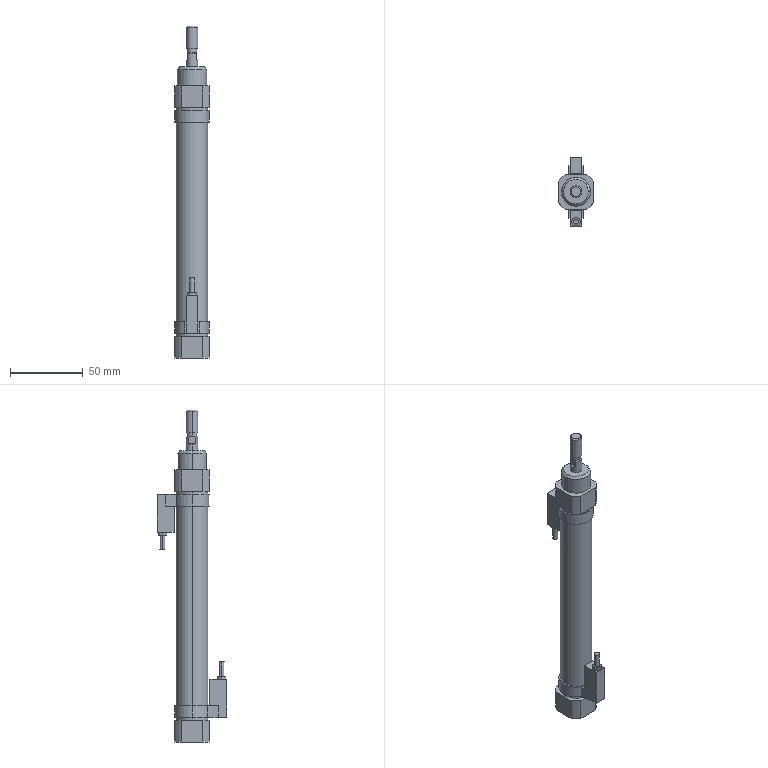Part | STEP file | Assembly electronic clip CDM2BZ20-125-C76(0) | 1 solid | 108 faces | box 24 x 47.6 x 228 mm | volume 84347 mm3 | plane 55 | cylinder 43 | cone 10 | commonest cylinder face diameters 23.6 x8 28 x8 21.6 x6 8 x5 3.4 x4 6 x4